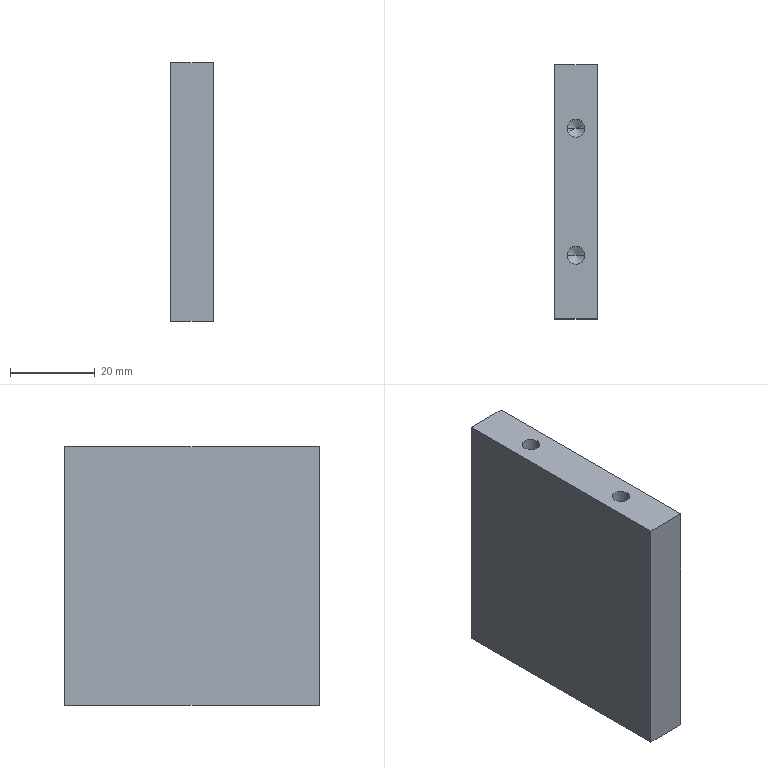Part | STEP file | 0232_207_Plate | 1 solid | 22 faces | box 10 x 60 x 61 mm | volume 35801 mm3 | cylinder 8 | cone 8 | plane 6 | commonest cylinder face diameters 4.2 x8
STEP:
#1=CARTESIAN_POINT('',(0.,0.,0.));
#2=DIRECTION('',(0.,0.,1.));
#3=DIRECTION('',(1.,0.,0.));
#4=AXIS2_PLACEMENT_3D('',#1,#2,#3);
#5=CARTESIAN_POINT('',(-7.1,15.,14.));
#6=VERTEX_POINT('',#5);
#7=CARTESIAN_POINT('',(-7.1,15.,0.));
#8=VERTEX_POINT('',#7);
#9=CARTESIAN_POINT('',(-7.1,15.,0.));
#10=DIRECTION('',(0.,0.,-1.));
#11=VECTOR('',#10,1.);
#12=LINE('',#9,#11);
#13=CARTESIAN_POINT('',(-5.,15.,0.));
#14=DIRECTION('',(0.,0.,-1.));
#15=DIRECTION('',(-1.,0.,0.));
#16=AXIS2_PLACEMENT_3D('',#13,#14,#15);
#17=CYLINDRICAL_SURFACE('',#16,2.1);
#18=CARTESIAN_POINT('',(6.283,0.));
#19=DIRECTION('',(0.,1.));
#20=VECTOR('',#19,1.);
#21=LINE('',#18,#20);
#22=(GEOMETRIC_REPRESENTATION_CONTEXT(2)PARAMETRIC_REPRESENTATION_CONTEXT()REPRESENTATION_CONTEXT('',''));
#23=DEFINITIONAL_REPRESENTATION('',(#21),#22);
#24=PCURVE('',#17,#23);
#25=CARTESIAN_POINT('',(-5.,15.,0.));
#26=DIRECTION('',(0.,0.,-1.));
#27=DIRECTION('',(-1.,0.,0.));
#28=AXIS2_PLACEMENT_3D('',#25,#26,#27);
#29=CYLINDRICAL_SURFACE('',#28,2.1);
#30=CARTESIAN_POINT('',(0.,0.));
#31=DIRECTION('',(0.,1.));
#32=VECTOR('',#31,1.);
#33=LINE('',#30,#32);
#34=(GEOMETRIC_REPRESENTATION_CONTEXT(2)PARAMETRIC_REPRESENTATION_CONTEXT()REPRESENTATION_CONTEXT('',''));
#35=DEFINITIONAL_REPRESENTATION('',(#33),#34);
#36=PCURVE('',#29,#35);
#37=SURFACE_CURVE('',#12,(#24,#36),.PCURVE_S1.);
#38=EDGE_CURVE('',#6,#8,#37,.T.);
#39=ORIENTED_EDGE('',*,*,#38,.T.);
#40=CARTESIAN_POINT('',(-2.9,15.,0.));
#41=VERTEX_POINT('',#40);
#42=CARTESIAN_POINT('',(-5.,15.,0.));
#43=DIRECTION('',(0.,0.,-1.));
#44=DIRECTION('',(-1.,0.,0.));
#45=AXIS2_PLACEMENT_3D('',#42,#43,#44);
#46=CIRCLE('',#45,2.1);
#47=CARTESIAN_POINT('',(0.,0.));
#48=DIRECTION('',(1.,0.));
#49=VECTOR('',#48,1.);
#50=LINE('',#47,#49);
#51=(GEOMETRIC_REPRESENTATION_CONTEXT(2)PARAMETRIC_REPRESENTATION_CONTEXT()REPRESENTATION_CONTEXT('',''));
#52=DEFINITIONAL_REPRESENTATION('',(#50),#51);
#53=PCURVE('',#17,#52);
#54=CARTESIAN_POINT('',(-10.,30.,0.));
#55=DIRECTION('',(0.,0.,-1.));
#56=DIRECTION('',(-1.,0.,0.));
#57=AXIS2_PLACEMENT_3D('',#54,#55,#56);
#58=PLANE('',#57);
#59=CARTESIAN_POINT('',(-5.,-15.));
#60=DIRECTION('',(1.,0.));
#61=AXIS2_PLACEMENT_2D('',#59,#60);
#62=CIRCLE('',#61,2.1);
#63=(GEOMETRIC_REPRESENTATION_CONTEXT(2)PARAMETRIC_REPRESENTATION_CONTEXT()REPRESENTATION_CONTEXT('',''));
#64=DEFINITIONAL_REPRESENTATION('',(#62),#63);
#65=PCURVE('',#58,#64);
#66=SURFACE_CURVE('',#46,(#53,#65),.PCURVE_S1.);
#67=EDGE_CURVE('',#41,#8,#66,.T.);
#68=ORIENTED_EDGE('',*,*,#67,.F.);
#69=CARTESIAN_POINT('',(-2.9,15.,14.));
#70=VERTEX_POINT('',#69);
#71=CARTESIAN_POINT('',(-2.9,15.,0.));
#72=DIRECTION('',(0.,0.,-1.));
#73=VECTOR('',#72,1.);
#74=LINE('',#71,#73);
#75=CARTESIAN_POINT('',(3.142,0.));
#76=DIRECTION('',(0.,1.));
#77=VECTOR('',#76,1.);
#78=LINE('',#75,#77);
#79=(GEOMETRIC_REPRESENTATION_CONTEXT(2)PARAMETRIC_REPRESENTATION_CONTEXT()REPRESENTATION_CONTEXT('',''));
#80=DEFINITIONAL_REPRESENTATION('',(#78),#79);
#81=PCURVE('',#17,#80);
#82=CARTESIAN_POINT('',(3.142,0.));
#83=DIRECTION('',(0.,1.));
#84=VECTOR('',#83,1.);
#85=LINE('',#82,#84);
#86=(GEOMETRIC_REPRESENTATION_CONTEXT(2)PARAMETRIC_REPRESENTATION_CONTEXT()REPRESENTATION_CONTEXT('',''));
#87=DEFINITIONAL_REPRESENTATION('',(#85),#86);
#88=PCURVE('',#29,#87);
#89=SURFACE_CURVE('',#74,(#81,#88),.PCURVE_S1.);
#90=EDGE_CURVE('',#70,#41,#89,.T.);
#91=ORIENTED_EDGE('',*,*,#90,.F.);
#92=CARTESIAN_POINT('',(-5.,15.,14.));
#93=DIRECTION('',(0.,0.,-1.));
#94=DIRECTION('',(-1.,0.,0.));
#95=AXIS2_PLACEMENT_3D('',#92,#93,#94);
#96=CIRCLE('',#95,2.1);
#97=CARTESIAN_POINT('',(0.,-14.));
#98=DIRECTION('',(1.,0.));
#99=VECTOR('',#98,1.);
#100=LINE('',#97,#99);
#101=(GEOMETRIC_REPRESENTATION_CONTEXT(2)PARAMETRIC_REPRESENTATION_CONTEXT()REPRESENTATION_CONTEXT('',''));
#102=DEFINITIONAL_REPRESENTATION('',(#100),#101);
#103=PCURVE('',#17,#102);
#104=CARTESIAN_POINT('',(-5.,15.,14.));
#105=DIRECTION('',(0.,0.,-1.));
#106=DIRECTION('',(-1.,0.,0.));
#107=AXIS2_PLACEMENT_3D('',#104,#105,#106);
#108=CONICAL_SURFACE('',#107,2.1,1.03);
#109=CARTESIAN_POINT('',(0.,0.));
#110=DIRECTION('',(1.,0.));
#111=VECTOR('',#110,1.);
#112=LINE('',#109,#111);
#113=(GEOMETRIC_REPRESENTATION_CONTEXT(2)PARAMETRIC_REPRESENTATION_CONTEXT()REPRESENTATION_CONTEXT('',''));
#114=DEFINITIONAL_REPRESENTATION('',(#112),#113);
#115=PCURVE('',#108,#114);
#116=SURFACE_CURVE('',#96,(#103,#115),.PCURVE_S1.);
#117=EDGE_CURVE('',#70,#6,#116,.T.);
#118=ORIENTED_EDGE('',*,*,#117,.T.);
#119=EDGE_LOOP('',(#39,#68,#91,#118));
#120=FACE_BOUND('',#119,.F.);
#121=ADVANCED_FACE('',(#120),#17,.F.);
#122=ORIENTED_EDGE('',*,*,#117,.F.);
#123=CARTESIAN_POINT('',(-5.,15.,15.262));
#124=VERTEX_POINT('',#123);
#125=CARTESIAN_POINT('',(-2.9,15.,14.));
#126=DIRECTION('',(0.8572,0.,-0.515));
#127=VECTOR('',#126,1.);
#128=LINE('',#125,#127);
#129=CARTESIAN_POINT('',(3.142,0.));
#130=DIRECTION('',(0.,1.));
#131=VECTOR('',#130,1.);
#132=LINE('',#129,#131);
#133=(GEOMETRIC_REPRESENTATION_CONTEXT(2)PARAMETRIC_REPRESENTATION_CONTEXT()REPRESENTATION_CONTEXT('',''));
#134=DEFINITIONAL_REPRESENTATION('',(#132),#133);
#135=PCURVE('',#108,#134);
#136=CARTESIAN_POINT('',(-5.,15.,14.));
#137=DIRECTION('',(0.,0.,-1.));
#138=DIRECTION('',(-1.,0.,0.));
#139=AXIS2_PLACEMENT_3D('',#136,#137,#138);
#140=CONICAL_SURFACE('',#139,2.1,1.03);
#141=CARTESIAN_POINT('',(3.142,0.));
#142=DIRECTION('',(0.,1.));
#143=VECTOR('',#142,1.);
#144=LINE('',#141,#143);
#145=(GEOMETRIC_REPRESENTATION_CONTEXT(2)PARAMETRIC_REPRESENTATION_CONTEXT()REPRESENTATION_CONTEXT('',''));
#146=DEFINITIONAL_REPRESENTATION('',(#144),#145);
#147=PCURVE('',#140,#146);
#148=SURFACE_CURVE('',#128,(#135,#147),.PCURVE_S1.);
#149=EDGE_CURVE('',#124,#70,#148,.T.);
#150=ORIENTED_EDGE('',*,*,#149,.F.);
#151=CARTESIAN_POINT('',(-7.1,15.,14.));
#152=DIRECTION('',(-0.8572,0.,-0.515));
#153=VECTOR('',#152,1.);
#154=LINE('',#151,#153);
#155=CARTESIAN_POINT('',(6.283,0.));
#156=DIRECTION('',(0.,1.));
#157=VECTOR('',#156,1.);
#158=LINE('',#155,#157);
#159=(GEOMETRIC_REPRESENTATION_CONTEXT(2)PARAMETRIC_REPRESENTATION_CONTEXT()REPRESENTATION_CONTEXT('',''));
#160=DEFINITIONAL_REPRESENTATION('',(#158),#159);
#161=PCURVE('',#108,#160);
#162=CARTESIAN_POINT('',(0.,0.));
#163=DIRECTION('',(0.,1.));
#164=VECTOR('',#163,1.);
#165=LINE('',#162,#164);
#166=(GEOMETRIC_REPRESENTATION_CONTEXT(2)PARAMETRIC_REPRESENTATION_CONTEXT()REPRESENTATION_CONTEXT('',''));
#167=DEFINITIONAL_REPRESENTATION('',(#165),#166);
#168=PCURVE('',#140,#167);
#169=SURFACE_CURVE('',#154,(#161,#168),.PCURVE_S1.);
#170=EDGE_CURVE('',#124,#6,#169,.T.);
#171=ORIENTED_EDGE('',*,*,#170,.T.);
#172=EDGE_LOOP('',(#122,#150,#171));
#173=FACE_BOUND('',#172,.F.);
#174=ADVANCED_FACE('',(#173),#108,.F.);
#175=CARTESIAN_POINT('',(-7.1,-15.,14.));
#176=VERTEX_POINT('',#175);
#177=CARTESIAN_POINT('',(-7.1,-15.,0.));
#178=VERTEX_POINT('',#177);
#179=CARTESIAN_POINT('',(-7.1,-15.,0.));
#180=DIRECTION('',(0.,0.,-1.));
#181=VECTOR('',#180,1.);
#182=LINE('',#179,#181);
#183=CARTESIAN_POINT('',(-5.,-15.,0.));
#184=DIRECTION('',(0.,0.,-1.));
#185=DIRECTION('',(-1.,0.,0.));
#186=AXIS2_PLACEMENT_3D('',#183,#184,#185);
#187=CYLINDRICAL_SURFACE('',#186,2.1);
#188=CARTESIAN_POINT('',(6.283,0.));
#189=DIRECTION('',(0.,1.));
#190=VECTOR('',#189,1.);
#191=LINE('',#188,#190);
#192=(GEOMETRIC_REPRESENTATION_CONTEXT(2)PARAMETRIC_REPRESENTATION_CONTEXT()REPRESENTATION_CONTEXT('',''));
#193=DEFINITIONAL_REPRESENTATION('',(#191),#192);
#194=PCURVE('',#187,#193);
#195=CARTESIAN_POINT('',(-5.,-15.,0.));
#196=DIRECTION('',(0.,0.,-1.));
#197=DIRECTION('',(-1.,0.,0.));
#198=AXIS2_PLACEMENT_3D('',#195,#196,#197);
#199=CYLINDRICAL_SURFACE('',#198,2.1);
#200=CARTESIAN_POINT('',(0.,0.));
#201=DIRECTION('',(0.,1.));
#202=VECTOR('',#201,1.);
#203=LINE('',#200,#202);
#204=(GEOMETRIC_REPRESENTATION_CONTEXT(2)PARAMETRIC_REPRESENTATION_CONTEXT()REPRESENTATION_CONTEXT('',''));
#205=DEFINITIONAL_REPRESENTATION('',(#203),#204);
#206=PCURVE('',#199,#205);
#207=SURFACE_CURVE('',#182,(#194,#206),.PCURVE_S1.);
#208=EDGE_CURVE('',#176,#178,#207,.T.);
#209=ORIENTED_EDGE('',*,*,#208,.T.);
#210=CARTESIAN_POINT('',(-2.9,-15.,0.));
#211=VERTEX_POINT('',#210);
#212=CARTESIAN_POINT('',(-5.,-15.,0.));
#213=DIRECTION('',(0.,0.,-1.));
#214=DIRECTION('',(-1.,0.,0.));
#215=AXIS2_PLACEMENT_3D('',#212,#213,#214);
#216=CIRCLE('',#215,2.1);
#217=CARTESIAN_POINT('',(0.,0.));
#218=DIRECTION('',(1.,0.));
#219=VECTOR('',#218,1.);
#220=LINE('',#217,#219);
#221=(GEOMETRIC_REPRESENTATION_CONTEXT(2)PARAMETRIC_REPRESENTATION_CONTEXT()REPRESENTATION_CONTEXT('',''));
#222=DEFINITIONAL_REPRESENTATION('',(#220),#221);
#223=PCURVE('',#187,#222);
#224=CARTESIAN_POINT('',(-5.,-45.));
#225=DIRECTION('',(1.,0.));
#226=AXIS2_PLACEMENT_2D('',#224,#225);
#227=CIRCLE('',#226,2.1);
#228=(GEOMETRIC_REPRESENTATION_CONTEXT(2)PARAMETRIC_REPRESENTATION_CONTEXT()REPRESENTATION_CONTEXT('',''));
#229=DEFINITIONAL_REPRESENTATION('',(#227),#228);
#230=PCURVE('',#58,#229);
#231=SURFACE_CURVE('',#216,(#223,#230),.PCURVE_S1.);
#232=EDGE_CURVE('',#211,#178,#231,.T.);
#233=ORIENTED_EDGE('',*,*,#232,.F.);
#234=CARTESIAN_POINT('',(-2.9,-15.,14.));
#235=VERTEX_POINT('',#234);
#236=CARTESIAN_POINT('',(-2.9,-15.,0.));
#237=DIRECTION('',(0.,0.,-1.));
#238=VECTOR('',#237,1.);
#239=LINE('',#236,#238);
#240=CARTESIAN_POINT('',(3.142,0.));
#241=DIRECTION('',(0.,1.));
#242=VECTOR('',#241,1.);
#243=LINE('',#240,#242);
#244=(GEOMETRIC_REPRESENTATION_CONTEXT(2)PARAMETRIC_REPRESENTATION_CONTEXT()REPRESENTATION_CONTEXT('',''));
#245=DEFINITIONAL_REPRESENTATION('',(#243),#244);
#246=PCURVE('',#187,#245);
#247=CARTESIAN_POINT('',(3.142,0.));
#248=DIRECTION('',(0.,1.));
#249=VECTOR('',#248,1.);
#250=LINE('',#247,#249);
#251=(GEOMETRIC_REPRESENTATION_CONTEXT(2)PARAMETRIC_REPRESENTATION_CONTEXT()REPRESENTATION_CONTEXT('',''));
#252=DEFINITIONAL_REPRESENTATION('',(#250),#251);
#253=PCURVE('',#199,#252);
#254=SURFACE_CURVE('',#239,(#246,#253),.PCURVE_S1.);
#255=EDGE_CURVE('',#235,#211,#254,.T.);
#256=ORIENTED_EDGE('',*,*,#255,.F.);
#257=CARTESIAN_POINT('',(-5.,-15.,14.));
#258=DIRECTION('',(0.,0.,-1.));
#259=DIRECTION('',(-1.,0.,0.));
#260=AXIS2_PLACEMENT_3D('',#257,#258,#259);
#261=CIRCLE('',#260,2.1);
#262=CARTESIAN_POINT('',(0.,-14.));
#263=DIRECTION('',(1.,0.));
#264=VECTOR('',#263,1.);
#265=LINE('',#262,#264);
#266=(GEOMETRIC_REPRESENTATION_CONTEXT(2)PARAMETRIC_REPRESENTATION_CONTEXT()REPRESENTATION_CONTEXT('',''));
#267=DEFINITIONAL_REPRESENTATION('',(#265),#266);
#268=PCURVE('',#187,#267);
#269=CARTESIAN_POINT('',(-5.,-15.,14.));
#270=DIRECTION('',(0.,0.,-1.));
#271=DIRECTION('',(-1.,0.,0.));
#272=AXIS2_PLACEMENT_3D('',#269,#270,#271);
#273=CONICAL_SURFACE('',#272,2.1,1.03);
#274=CARTESIAN_POINT('',(0.,0.));
#275=DIRECTION('',(1.,0.));
#276=VECTOR('',#275,1.);
#277=LINE('',#274,#276);
#278=(GEOMETRIC_REPRESENTATION_CONTEXT(2)PARAMETRIC_REPRESENTATION_CONTEXT()REPRESENTATION_CONTEXT('',''));
#279=DEFINITIONAL_REPRESENTATION('',(#277),#278);
#280=PCURVE('',#273,#279);
#281=SURFACE_CURVE('',#261,(#268,#280),.PCURVE_S1.);
#282=EDGE_CURVE('',#235,#176,#281,.T.);
#283=ORIENTED_EDGE('',*,*,#282,.T.);
#284=EDGE_LOOP('',(#209,#233,#256,#283));
#285=FACE_BOUND('',#284,.F.);
#286=ADVANCED_FACE('',(#285),#187,.F.);
#287=ORIENTED_EDGE('',*,*,#282,.F.);
#288=CARTESIAN_POINT('',(-5.,-15.,15.262));
#289=VERTEX_POINT('',#288);
#290=CARTESIAN_POINT('',(-2.9,-15.,14.));
#291=DIRECTION('',(0.8572,0.,-0.515));
#292=VECTOR('',#291,1.);
#293=LINE('',#290,#292);
#294=CARTESIAN_POINT('',(3.142,0.));
#295=DIRECTION('',(0.,1.));
#296=VECTOR('',#295,1.);
#297=LINE('',#294,#296);
#298=(GEOMETRIC_REPRESENTATION_CONTEXT(2)PARAMETRIC_REPRESENTATION_CONTEXT()REPRESENTATION_CONTEXT('',''));
#299=DEFINITIONAL_REPRESENTATION('',(#297),#298);
#300=PCURVE('',#273,#299);
#301=CARTESIAN_POINT('',(-5.,-15.,14.));
#302=DIRECTION('',(0.,0.,-1.));
#303=DIRECTION('',(-1.,0.,0.));
#304=AXIS2_PLACEMENT_3D('',#301,#302,#303);
#305=CONICAL_SURFACE('',#304,2.1,1.03);
#306=CARTESIAN_POINT('',(3.142,0.));
#307=DIRECTION('',(0.,1.));
#308=VECTOR('',#307,1.);
#309=LINE('',#306,#308);
#310=(GEOMETRIC_REPRESENTATION_CONTEXT(2)PARAMETRIC_REPRESENTATION_CONTEXT()REPRESENTATION_CONTEXT('',''));
#311=DEFINITIONAL_REPRESENTATION('',(#309),#310);
#312=PCURVE('',#305,#311);
#313=SURFACE_CURVE('',#293,(#300,#312),.PCURVE_S1.);
#314=EDGE_CURVE('',#289,#235,#313,.T.);
#315=ORIENTED_EDGE('',*,*,#314,.F.);
#316=CARTESIAN_POINT('',(-7.1,-15.,14.));
#317=DIRECTION('',(-0.8572,0.,-0.515));
#318=VECTOR('',#317,1.);
#319=LINE('',#316,#318);
#320=CARTESIAN_POINT('',(6.283,0.));
#321=DIRECTION('',(0.,1.));
#322=VECTOR('',#321,1.);
#323=LINE('',#320,#322);
#324=(GEOMETRIC_REPRESENTATION_CONTEXT(2)PARAMETRIC_REPRESENTATION_CONTEXT()REPRESENTATION_CONTEXT('',''));
#325=DEFINITIONAL_REPRESENTATION('',(#323),#324);
#326=PCURVE('',#273,#325);
#327=CARTESIAN_POINT('',(0.,0.));
#328=DIRECTION('',(0.,1.));
#329=VECTOR('',#328,1.);
#330=LINE('',#327,#329);
#331=(GEOMETRIC_REPRESENTATION_CONTEXT(2)PARAMETRIC_REPRESENTATION_CONTEXT()REPRESENTATION_CONTEXT('',''));
#332=DEFINITIONAL_REPRESENTATION('',(#330),#331);
#333=PCURVE('',#305,#332);
#334=SURFACE_CURVE('',#319,(#326,#333),.PCURVE_S1.);
#335=EDGE_CURVE('',#289,#176,#334,.T.);
#336=ORIENTED_EDGE('',*,*,#335,.T.);
#337=EDGE_LOOP('',(#287,#315,#336));
#338=FACE_BOUND('',#337,.F.);
#339=ADVANCED_FACE('',(#338),#273,.F.);
#340=CARTESIAN_POINT('',(-2.9,-15.,47.));
#341=VERTEX_POINT('',#340);
#342=CARTESIAN_POINT('',(-2.9,-15.,61.));
#343=VERTEX_POINT('',#342);
#344=CARTESIAN_POINT('',(-2.9,-15.,61.));
#345=DIRECTION('',(0.,0.,1.));
#346=VECTOR('',#345,1.);
#347=LINE('',#344,#346);
#348=CARTESIAN_POINT('',(-5.,-15.,61.));
#349=DIRECTION('',(0.,0.,1.));
#350=DIRECTION('',(1.,0.,0.));
#351=AXIS2_PLACEMENT_3D('',#348,#349,#350);
#352=CYLINDRICAL_SURFACE('',#351,2.1);
#353=CARTESIAN_POINT('',(6.283,0.));
#354=DIRECTION('',(0.,1.));
#355=VECTOR('',#354,1.);
#356=LINE('',#353,#355);
#357=(GEOMETRIC_REPRESENTATION_CONTEXT(2)PARAMETRIC_REPRESENTATION_CONTEXT()REPRESENTATION_CONTEXT('',''));
#358=DEFINITIONAL_REPRESENTATION('',(#356),#357);
#359=PCURVE('',#352,#358);
#360=CARTESIAN_POINT('',(-5.,-15.,61.));
#361=DIRECTION('',(0.,0.,1.));
#362=DIRECTION('',(1.,0.,0.));
#363=AXIS2_PLACEMENT_3D('',#360,#361,#362);
#364=CYLINDRICAL_SURFACE('',#363,2.1);
#365=CARTESIAN_POINT('',(0.,0.));
#366=DIRECTION('',(0.,1.));
#367=VECTOR('',#366,1.);
#368=LINE('',#365,#367);
#369=(GEOMETRIC_REPRESENTATION_CONTEXT(2)PARAMETRIC_REPRESENTATION_CONTEXT()REPRESENTATION_CONTEXT('',''));
#370=DEFINITIONAL_REPRESENTATION('',(#368),#369);
#371=PCURVE('',#364,#370);
#372=SURFACE_CURVE('',#347,(#359,#371),.PCURVE_S1.);
#373=EDGE_CURVE('',#341,#343,#372,.T.);
#374=ORIENTED_EDGE('',*,*,#373,.T.);
#375=CARTESIAN_POINT('',(-7.1,-15.,61.));
#376=VERTEX_POINT('',#375);
#377=CARTESIAN_POINT('',(-5.,-15.,61.));
#378=DIRECTION('',(0.,0.,1.));
#379=DIRECTION('',(1.,0.,0.));
#380=AXIS2_PLACEMENT_3D('',#377,#378,#379);
#381=CIRCLE('',#380,2.1);
#382=CARTESIAN_POINT('',(0.,0.));
#383=DIRECTION('',(1.,0.));
#384=VECTOR('',#383,1.);
#385=LINE('',#382,#384);
#386=(GEOMETRIC_REPRESENTATION_CONTEXT(2)PARAMETRIC_REPRESENTATION_CONTEXT()REPRESENTATION_CONTEXT('',''));
#387=DEFINITIONAL_REPRESENTATION('',(#385),#386);
#388=PCURVE('',#352,#387);
#389=CARTESIAN_POINT('',(-10.,30.,61.));
#390=DIRECTION('',(0.,0.,1.));
#391=DIRECTION('',(1.,0.,0.));
#392=AXIS2_PLACEMENT_3D('',#389,#390,#391);
#393=PLANE('',#392);
#394=CARTESIAN_POINT('',(5.,-45.));
#395=DIRECTION('',(1.,0.));
#396=AXIS2_PLACEMENT_2D('',#394,#395);
#397=CIRCLE('',#396,2.1);
#398=(GEOMETRIC_REPRESENTATION_CONTEXT(2)PARAMETRIC_REPRESENTATION_CONTEXT()REPRESENTATION_CONTEXT('',''));
#399=DEFINITIONAL_REPRESENTATION('',(#397),#398);
#400=PCURVE('',#393,#399);
#401=SURFACE_CURVE('',#381,(#388,#400),.PCURVE_S1.);
#402=EDGE_CURVE('',#376,#343,#401,.T.);
#403=ORIENTED_EDGE('',*,*,#402,.F.);
#404=CARTESIAN_POINT('',(-7.1,-15.,47.));
#405=VERTEX_POINT('',#404);
#406=CARTESIAN_POINT('',(-7.1,-15.,61.));
#407=DIRECTION('',(0.,0.,1.));
#408=VECTOR('',#407,1.);
#409=LINE('',#406,#408);
#410=CARTESIAN_POINT('',(3.142,0.));
#411=DIRECTION('',(0.,1.));
#412=VECTOR('',#411,1.);
#413=LINE('',#410,#412);
#414=(GEOMETRIC_REPRESENTATION_CONTEXT(2)PARAMETRIC_REPRESENTATION_CONTEXT()REPRESENTATION_CONTEXT('',''));
#415=DEFINITIONAL_REPRESENTATION('',(#413),#414);
#416=PCURVE('',#352,#415);
#417=CARTESIAN_POINT('',(3.142,0.));
#418=DIRECTION('',(0.,1.));
#419=VECTOR('',#418,1.);
#420=LINE('',#417,#419);
#421=(GEOMETRIC_REPRESENTATION_CONTEXT(2)PARAMETRIC_REPRESENTATION_CONTEXT()REPRESENTATION_CONTEXT('',''));
#422=DEFINITIONAL_REPRESENTATION('',(#420),#421);
#423=PCURVE('',#364,#422);
#424=SURFACE_CURVE('',#409,(#416,#423),.PCURVE_S1.);
#425=EDGE_CURVE('',#405,#376,#424,.T.);
#426=ORIENTED_EDGE('',*,*,#425,.F.);
#427=CARTESIAN_POINT('',(-5.,-15.,47.));
#428=DIRECTION('',(0.,0.,1.));
#429=DIRECTION('',(1.,0.,0.));
#430=AXIS2_PLACEMENT_3D('',#427,#428,#429);
#431=CIRCLE('',#430,2.1);
#432=CARTESIAN_POINT('',(0.,-14.));
#433=DIRECTION('',(1.,0.));
#434=VECTOR('',#433,1.);
#435=LINE('',#432,#434);
#436=(GEOMETRIC_REPRESENTATION_CONTEXT(2)PARAMETRIC_REPRESENTATION_CONTEXT()REPRESENTATION_CONTEXT('',''));
#437=DEFINITIONAL_REPRESENTATION('',(#435),#436);
#438=PCURVE('',#352,#437);
#439=CARTESIAN_POINT('',(-5.,-15.,47.));
#440=DIRECTION('',(0.,0.,1.));
#441=DIRECTION('',(1.,0.,0.));
#442=AXIS2_PLACEMENT_3D('',#439,#440,#441);
#443=CONICAL_SURFACE('',#442,2.1,1.03);
#444=CARTESIAN_POINT('',(0.,0.));
#445=DIRECTION('',(1.,0.));
#446=VECTOR('',#445,1.);
#447=LINE('',#444,#446);
#448=(GEOMETRIC_REPRESENTATION_CONTEXT(2)PARAMETRIC_REPRESENTATION_CONTEXT()REPRESENTATION_CONTEXT('',''));
#449=DEFINITIONAL_REPRESENTATION('',(#447),#448);
#450=PCURVE('',#443,#449);
#451=SURFACE_CURVE('',#431,(#438,#450),.PCURVE_S1.);
#452=EDGE_CURVE('',#405,#341,#451,.T.);
#453=ORIENTED_EDGE('',*,*,#452,.T.);
#454=EDGE_LOOP('',(#374,#403,#426,#453));
#455=FACE_BOUND('',#454,.F.);
#456=ADVANCED_FACE('',(#455),#352,.F.);
#457=ORIENTED_EDGE('',*,*,#452,.F.);
#458=CARTESIAN_POINT('',(-5.,-15.,45.738));
#459=VERTEX_POINT('',#458);
#460=CARTESIAN_POINT('',(-7.1,-15.,47.));
#461=DIRECTION('',(-0.8572,0.,0.515));
#462=VECTOR('',#461,1.);
#463=LINE('',#460,#462);
#464=CARTESIAN_POINT('',(3.142,0.));
#465=DIRECTION('',(0.,1.));
#466=VECTOR('',#465,1.);
#467=LINE('',#464,#466);
#468=(GEOMETRIC_REPRESENTATION_CONTEXT(2)PARAMETRIC_REPRESENTATION_CONTEXT()REPRESENTATION_CONTEXT('',''));
#469=DEFINITIONAL_REPRESENTATION('',(#467),#468);
#470=PCURVE('',#443,#469);
#471=CARTESIAN_POINT('',(-5.,-15.,47.));
#472=DIRECTION('',(0.,0.,1.));
#473=DIRECTION('',(1.,0.,0.));
#474=AXIS2_PLACEMENT_3D('',#471,#472,#473);
#475=CONICAL_SURFACE('',#474,2.1,1.03);
#476=CARTESIAN_POINT('',(3.142,0.));
#477=DIRECTION('',(0.,1.));
#478=VECTOR('',#477,1.);
#479=LINE('',#476,#478);
#480=(GEOMETRIC_REPRESENTATION_CONTEXT(2)PARAMETRIC_REPRESENTATION_CONTEXT()REPRESENTATION_CONTEXT('',''));
#481=DEFINITIONAL_REPRESENTATION('',(#479),#480);
#482=PCURVE('',#475,#481);
#483=SURFACE_CURVE('',#463,(#470,#482),.PCURVE_S1.);
#484=EDGE_CURVE('',#459,#405,#483,.T.);
#485=ORIENTED_EDGE('',*,*,#484,.F.);
#486=CARTESIAN_POINT('',(-2.9,-15.,47.));
#487=DIRECTION('',(0.8572,0.,0.515));
#488=VECTOR('',#487,1.);
#489=LINE('',#486,#488);
#490=CARTESIAN_POINT('',(6.283,0.));
#491=DIRECTION('',(0.,1.));
#492=VECTOR('',#491,1.);
#493=LINE('',#490,#492);
#494=(GEOMETRIC_REPRESENTATION_CONTEXT(2)PARAMETRIC_REPRESENTATION_CONTEXT()REPRESENTATION_CONTEXT('',''));
#495=DEFINITIONAL_REPRESENTATION('',(#493),#494);
#496=PCURVE('',#443,#495);
#497=CARTESIAN_POINT('',(0.,0.));
#498=DIRECTION('',(0.,1.));
#499=VECTOR('',#498,1.);
#500=LINE('',#497,#499);
#501=(GEOMETRIC_REPRESENTATION_CONTEXT(2)PARAMETRIC_REPRESENTATION_CONTEXT()REPRESENTATION_CONTEXT('',''));
#502=DEFINITIONAL_REPRESENTATION('',(#500),#501);
#503=PCURVE('',#475,#502);
#504=SURFACE_CURVE('',#489,(#496,#503),.PCURVE_S1.);
#505=EDGE_CURVE('',#459,#341,#504,.T.);
#506=ORIENTED_EDGE('',*,*,#505,.T.);
#507=EDGE_LOOP('',(#457,#485,#506));
#508=FACE_BOUND('',#507,.F.);
#509=ADVANCED_FACE('',(#508),#443,.F.);
#510=CARTESIAN_POINT('',(-2.9,15.,47.));
#511=VERTEX_POINT('',#510);
#512=CARTESIAN_POINT('',(-2.9,15.,61.));
#513=VERTEX_POINT('',#512);
#514=CARTESIAN_POINT('',(-2.9,15.,61.));
#515=DIRECTION('',(0.,0.,1.));
#516=VECTOR('',#515,1.);
#517=LINE('',#514,#516);
#518=CARTESIAN_POINT('',(-5.,15.,61.));
#519=DIRECTION('',(0.,0.,1.));
#520=DIRECTION('',(1.,0.,0.));
#521=AXIS2_PLACEMENT_3D('',#518,#519,#520);
#522=CYLINDRICAL_SURFACE('',#521,2.1);
#523=CARTESIAN_POINT('',(6.283,0.));
#524=DIRECTION('',(0.,1.));
#525=VECTOR('',#524,1.);
#526=LINE('',#523,#525);
#527=(GEOMETRIC_REPRESENTATION_CONTEXT(2)PARAMETRIC_REPRESENTATION_CONTEXT()REPRESENTATION_CONTEXT('',''));
#528=DEFINITIONAL_REPRESENTATION('',(#526),#527);
#529=PCURVE('',#522,#528);
#530=CARTESIAN_POINT('',(-5.,15.,61.));
#531=DIRECTION('',(0.,0.,1.));
#532=DIRECTION('',(1.,0.,0.));
#533=AXIS2_PLACEMENT_3D('',#530,#531,#532);
#534=CYLINDRICAL_SURFACE('',#533,2.1);
#535=CARTESIAN_POINT('',(0.,0.));
#536=DIRECTION('',(0.,1.));
#537=VECTOR('',#536,1.);
#538=LINE('',#535,#537);
#539=(GEOMETRIC_REPRESENTATION_CONTEXT(2)PARAMETRIC_REPRESENTATION_CONTEXT()REPRESENTATION_CONTEXT('',''));
#540=DEFINITIONAL_REPRESENTATION('',(#538),#539);
#541=PCURVE('',#534,#540);
#542=SURFACE_CURVE('',#517,(#529,#541),.PCURVE_S1.);
#543=EDGE_CURVE('',#511,#513,#542,.T.);
#544=ORIENTED_EDGE('',*,*,#543,.T.);
#545=CARTESIAN_POINT('',(-7.1,15.,61.));
#546=VERTEX_POINT('',#545);
#547=CARTESIAN_POINT('',(-5.,15.,61.));
#548=DIRECTION('',(0.,0.,1.));
#549=DIRECTION('',(1.,0.,0.));
#550=AXIS2_PLACEMENT_3D('',#547,#548,#549);
#551=CIRCLE('',#550,2.1);
#552=CARTESIAN_POINT('',(0.,0.));
#553=DIRECTION('',(1.,0.));
#554=VECTOR('',#553,1.);
#555=LINE('',#552,#554);
#556=(GEOMETRIC_REPRESENTATION_CONTEXT(2)PARAMETRIC_REPRESENTATION_CONTEXT()REPRESENTATION_CONTEXT('',''));
#557=DEFINITIONAL_REPRESENTATION('',(#555),#556);
#558=PCURVE('',#522,#557);
#559=CARTESIAN_POINT('',(5.,-15.));
#560=DIRECTION('',(1.,0.));
#561=AXIS2_PLACEMENT_2D('',#559,#560);
#562=CIRCLE('',#561,2.1);
#563=(GEOMETRIC_REPRESENTATION_CONTEXT(2)PARAMETRIC_REPRESENTATION_CONTEXT()REPRESENTATION_CONTEXT('',''));
#564=DEFINITIONAL_REPRESENTATION('',(#562),#563);
#565=PCURVE('',#393,#564);
#566=SURFACE_CURVE('',#551,(#558,#565),.PCURVE_S1.);
#567=EDGE_CURVE('',#546,#513,#566,.T.);
#568=ORIENTED_EDGE('',*,*,#567,.F.);
#569=CARTESIAN_POINT('',(-7.1,15.,47.));
#570=VERTEX_POINT('',#569);
#571=CARTESIAN_POINT('',(-7.1,15.,61.));
#572=DIRECTION('',(0.,0.,1.));
#573=VECTOR('',#572,1.);
#574=LINE('',#571,#573);
#575=CARTESIAN_POINT('',(3.142,0.));
#576=DIRECTION('',(0.,1.));
#577=VECTOR('',#576,1.);
#578=LINE('',#575,#577);
#579=(GEOMETRIC_REPRESENTATION_CONTEXT(2)PARAMETRIC_REPRESENTATION_CONTEXT()REPRESENTATION_CONTEXT('',''));
#580=DEFINITIONAL_REPRESENTATION('',(#578),#579);
#581=PCURVE('',#522,#580);
#582=CARTESIAN_POINT('',(3.142,0.));
#583=DIRECTION('',(0.,1.));
#584=VECTOR('',#583,1.);
#585=LINE('',#582,#584);
#586=(GEOMETRIC_REPRESENTATION_CONTEXT(2)PARAMETRIC_REPRESENTATION_CONTEXT()REPRESENTATION_CONTEXT('',''));
#587=DEFINITIONAL_REPRESENTATION('',(#585),#586);
#588=PCURVE('',#534,#587);
#589=SURFACE_CURVE('',#574,(#581,#588),.PCURVE_S1.);
#590=EDGE_CURVE('',#570,#546,#589,.T.);
#591=ORIENTED_EDGE('',*,*,#590,.F.);
#592=CARTESIAN_POINT('',(-5.,15.,47.));
#593=DIRECTION('',(0.,0.,1.));
#594=DIRECTION('',(1.,0.,0.));
#595=AXIS2_PLACEMENT_3D('',#592,#593,#594);
#596=CIRCLE('',#595,2.1);
#597=CARTESIAN_POINT('',(0.,-14.));
#598=DIRECTION('',(1.,0.));
#599=VECTOR('',#598,1.);
#600=LINE('',#597,#599);
#601=(GEOMETRIC_REPRESENTATION_CONTEXT(2)PARAMETRIC_REPRESENTATION_CONTEXT()REPRESENTATION_CONTEXT('',''));
#602=DEFINITIONAL_REPRESENTATION('',(#600),#601);
#603=PCURVE('',#522,#602);
#604=CARTESIAN_POINT('',(-5.,15.,47.));
#605=DIRECTION('',(0.,0.,1.));
#606=DIRECTION('',(1.,0.,0.));
#607=AXIS2_PLACEMENT_3D('',#604,#605,#606);
#608=CONICAL_SURFACE('',#607,2.1,1.03);
#609=CARTESIAN_POINT('',(0.,0.));
#610=DIRECTION('',(1.,0.));
#611=VECTOR('',#610,1.);
#612=LINE('',#609,#611);
#613=(GEOMETRIC_REPRESENTATION_CONTEXT(2)PARAMETRIC_REPRESENTATION_CONTEXT()REPRESENTATION_CONTEXT('',''));
#614=DEFINITIONAL_REPRESENTATION('',(#612),#613);
#615=PCURVE('',#608,#614);
#616=SURFACE_CURVE('',#596,(#603,#615),.PCURVE_S1.);
#617=EDGE_CURVE('',#570,#511,#616,.T.);
#618=ORIENTED_EDGE('',*,*,#617,.T.);
#619=EDGE_LOOP('',(#544,#568,#591,#618));
#620=FACE_BOUND('',#619,.F.);
#621=ADVANCED_FACE('',(#620),#522,.F.);
#622=ORIENTED_EDGE('',*,*,#617,.F.);
#623=CARTESIAN_POINT('',(-5.,15.,45.738));
#624=VERTEX_POINT('',#623);
#625=CARTESIAN_POINT('',(-7.1,15.,47.));
#626=DIRECTION('',(-0.8572,0.,0.515));
#627=VECTOR('',#626,1.);
#628=LINE('',#625,#627);
#629=CARTESIAN_POINT('',(3.142,0.));
#630=DIRECTION('',(0.,1.));
#631=VECTOR('',#630,1.);
#632=LINE('',#629,#631);
#633=(GEOMETRIC_REPRESENTATION_CONTEXT(2)PARAMETRIC_REPRESENTATION_CONTEXT()REPRESENTATION_CONTEXT('',''));
#634=DEFINITIONAL_REPRESENTATION('',(#632),#633);
#635=PCURVE('',#608,#634);
#636=CARTESIAN_POINT('',(-5.,15.,47.));
#637=DIRECTION('',(0.,0.,1.));
#638=DIRECTION('',(1.,0.,0.));
#639=AXIS2_PLACEMENT_3D('',#636,#637,#638);
#640=CONICAL_SURFACE('',#639,2.1,1.03);
#641=CARTESIAN_POINT('',(3.142,0.));
#642=DIRECTION('',(0.,1.));
#643=VECTOR('',#642,1.);
#644=LINE('',#641,#643);
#645=(GEOMETRIC_REPRESENTATION_CONTEXT(2)PARAMETRIC_REPRESENTATION_CONTEXT()REPRESENTATION_CONTEXT('',''));
#646=DEFINITIONAL_REPRESENTATION('',(#644),#645);
#647=PCURVE('',#640,#646);
#648=SURFACE_CURVE('',#628,(#635,#647),.PCURVE_S1.);
#649=EDGE_CURVE('',#624,#570,#648,.T.);
#650=ORIENTED_EDGE('',*,*,#649,.F.);
#651=CARTESIAN_POINT('',(-2.9,15.,47.));
#652=DIRECTION('',(0.8572,0.,0.515));
#653=VECTOR('',#652,1.);
#654=LINE('',#651,#653);
#655=CARTESIAN_POINT('',(6.283,0.));
#656=DIRECTION('',(0.,1.));
#657=VECTOR('',#656,1.);
#658=LINE('',#655,#657);
#659=(GEOMETRIC_REPRESENTATION_CONTEXT(2)PARAMETRIC_REPRESENTATION_CONTEXT()REPRESENTATION_CONTEXT('',''));
#660=DEFINITIONAL_REPRESENTATION('',(#658),#659);
#661=PCURVE('',#608,#660);
#662=CARTESIAN_POINT('',(0.,0.));
#663=DIRECTION('',(0.,1.));
#664=VECTOR('',#663,1.);
#665=LINE('',#662,#664);
#666=(GEOMETRIC_REPRESENTATION_CONTEXT(2)PARAMETRIC_REPRESENTATION_CONTEXT()REPRESENTATION_CONTEXT('',''));
#667=DEFINITIONAL_REPRESENTATION('',(#665),#666);
#668=PCURVE('',#640,#667);
#669=SURFACE_CURVE('',#654,(#661,#668),.PCURVE_S1.);
#670=EDGE_CURVE('',#624,#511,#669,.T.);
#671=ORIENTED_EDGE('',*,*,#670,.T.);
#672=EDGE_LOOP('',(#622,#650,#671));
#673=FACE_BOUND('',#672,.F.);
#674=ADVANCED_FACE('',(#673),#608,.F.);
#675=CARTESIAN_POINT('',(-5.,-15.,61.));
#676=DIRECTION('',(0.,0.,1.));
#677=DIRECTION('',(1.,0.,0.));
#678=AXIS2_PLACEMENT_3D('',#675,#676,#677);
#679=CIRCLE('',#678,2.1);
#680=CARTESIAN_POINT('',(5.,-45.));
#681=DIRECTION('',(1.,0.));
#682=AXIS2_PLACEMENT_2D('',#680,#681);
#683=CIRCLE('',#682,2.1);
#684=(GEOMETRIC_REPRESENTATION_CONTEXT(2)PARAMETRIC_REPRESENTATION_CONTEXT()REPRESENTATION_CONTEXT('',''));
#685=DEFINITIONAL_REPRESENTATION('',(#683),#684);
#686=PCURVE('',#393,#685);
#687=CARTESIAN_POINT('',(0.,0.));
#688=DIRECTION('',(1.,0.));
#689=VECTOR('',#688,1.);
#690=LINE('',#687,#689);
#691=(GEOMETRIC_REPRESENTATION_CONTEXT(2)PARAMETRIC_REPRESENTATION_CONTEXT()REPRESENTATION_CONTEXT('',''));
#692=DEFINITIONAL_REPRESENTATION('',(#690),#691);
#693=PCURVE('',#364,#692);
#694=SURFACE_CURVE('',#679,(#686,#693),.PCURVE_S1.);
#695=EDGE_CURVE('',#343,#376,#694,.T.);
#696=ORIENTED_EDGE('',*,*,#695,.F.);
#697=ORIENTED_EDGE('',*,*,#402,.F.);
#698=EDGE_LOOP('',(#696,#697));
#699=FACE_BOUND('',#698,.T.);
#700=CARTESIAN_POINT('',(-5.,15.,61.));
#701=DIRECTION('',(0.,0.,1.));
#702=DIRECTION('',(1.,0.,0.));
#703=AXIS2_PLACEMENT_3D('',#700,#701,#702);
#704=CIRCLE('',#703,2.1);
#705=CARTESIAN_POINT('',(5.,-15.));
#706=DIRECTION('',(1.,0.));
#707=AXIS2_PLACEMENT_2D('',#705,#706);
#708=CIRCLE('',#707,2.1);
#709=(GEOMETRIC_REPRESENTATION_CONTEXT(2)PARAMETRIC_REPRESENTATION_CONTEXT()REPRESENTATION_CONTEXT('',''));
#710=DEFINITIONAL_REPRESENTATION('',(#708),#709);
#711=PCURVE('',#393,#710);
#712=CARTESIAN_POINT('',(0.,0.));
#713=DIRECTION('',(1.,0.));
#714=VECTOR('',#713,1.);
#715=LINE('',#712,#714);
#716=(GEOMETRIC_REPRESENTATION_CONTEXT(2)PARAMETRIC_REPRESENTATION_CONTEXT()REPRESENTATION_CONTEXT('',''));
#717=DEFINITIONAL_REPRESENTATION('',(#715),#716);
#718=PCURVE('',#534,#717);
#719=SURFACE_CURVE('',#704,(#711,#718),.PCURVE_S1.);
#720=EDGE_CURVE('',#513,#546,#719,.T.);
#721=ORIENTED_EDGE('',*,*,#720,.F.);
#722=ORIENTED_EDGE('',*,*,#567,.F.);
#723=EDGE_LOOP('',(#721,#722));
#724=FACE_BOUND('',#723,.T.);
#725=CARTESIAN_POINT('',(0.,30.,61.));
#726=VERTEX_POINT('',#725);
#727=CARTESIAN_POINT('',(0.,-30.,61.));
#728=VERTEX_POINT('',#727);
#729=CARTESIAN_POINT('',(0.,30.,61.));
#730=DIRECTION('',(0.,-1.,0.));
#731=VECTOR('',#730,1.);
#732=LINE('',#729,#731);
#733=CARTESIAN_POINT('',(10.,0.));
#734=DIRECTION('',(0.,-1.));
#735=VECTOR('',#734,1.);
#736=LINE('',#733,#735);
#737=(GEOMETRIC_REPRESENTATION_CONTEXT(2)PARAMETRIC_REPRESENTATION_CONTEXT()REPRESENTATION_CONTEXT('',''));
#738=DEFINITIONAL_REPRESENTATION('',(#736),#737);
#739=PCURVE('',#393,#738);
#740=CARTESIAN_POINT('',(0.,-30.,61.));
#741=DIRECTION('',(1.,0.,0.));
#742=DIRECTION('',(0.,0.,-1.));
#743=AXIS2_PLACEMENT_3D('',#740,#741,#742);
#744=PLANE('',#743);
#745=CARTESIAN_POINT('',(0.,60.));
#746=DIRECTION('',(0.,-1.));
#747=VECTOR('',#746,1.);
#748=LINE('',#745,#747);
#749=(GEOMETRIC_REPRESENTATION_CONTEXT(2)PARAMETRIC_REPRESENTATION_CONTEXT()REPRESENTATION_CONTEXT('',''));
#750=DEFINITIONAL_REPRESENTATION('',(#748),#749);
#751=PCURVE('',#744,#750);
#752=SURFACE_CURVE('',#732,(#739,#751),.PCURVE_S1.);
#753=EDGE_CURVE('',#726,#728,#752,.T.);
#754=ORIENTED_EDGE('',*,*,#753,.F.);
#755=CARTESIAN_POINT('',(-10.,30.,61.));
#756=VERTEX_POINT('',#755);
#757=CARTESIAN_POINT('',(-10.,30.,61.));
#758=DIRECTION('',(1.,0.,0.));
#759=VECTOR('',#758,1.);
#760=LINE('',#757,#759);
#761=CARTESIAN_POINT('',(0.,0.));
#762=DIRECTION('',(1.,0.));
#763=VECTOR('',#762,1.);
#764=LINE('',#761,#763);
#765=(GEOMETRIC_REPRESENTATION_CONTEXT(2)PARAMETRIC_REPRESENTATION_CONTEXT()REPRESENTATION_CONTEXT('',''));
#766=DEFINITIONAL_REPRESENTATION('',(#764),#765);
#767=PCURVE('',#393,#766);
#768=CARTESIAN_POINT('',(-10.,30.,61.));
#769=DIRECTION('',(0.,1.,0.));
#770=DIRECTION('',(0.,0.,1.));
#771=AXIS2_PLACEMENT_3D('',#768,#769,#770);
#772=PLANE('',#771);
#773=CARTESIAN_POINT('',(0.,0.));
#774=DIRECTION('',(0.,1.));
#775=VECTOR('',#774,1.);
#776=LINE('',#773,#775);
#777=(GEOMETRIC_REPRESENTATION_CONTEXT(2)PARAMETRIC_REPRESENTATION_CONTEXT()REPRESENTATION_CONTEXT('',''));
#778=DEFINITIONAL_REPRESENTATION('',(#776),#777);
#779=PCURVE('',#772,#778);
#780=SURFACE_CURVE('',#760,(#767,#779),.PCURVE_S1.);
#781=EDGE_CURVE('',#756,#726,#780,.T.);
#782=ORIENTED_EDGE('',*,*,#781,.F.);
#783=CARTESIAN_POINT('',(-10.,-30.,61.));
#784=VERTEX_POINT('',#783);
#785=CARTESIAN_POINT('',(-10.,30.,61.));
#786=DIRECTION('',(0.,-1.,0.));
#787=VECTOR('',#786,1.);
#788=LINE('',#785,#787);
#789=CARTESIAN_POINT('',(0.,0.));
#790=DIRECTION('',(0.,-1.));
#791=VECTOR('',#790,1.);
#792=LINE('',#789,#791);
#793=(GEOMETRIC_REPRESENTATION_CONTEXT(2)PARAMETRIC_REPRESENTATION_CONTEXT()REPRESENTATION_CONTEXT('',''));
#794=DEFINITIONAL_REPRESENTATION('',(#792),#793);
#795=PCURVE('',#393,#794);
#796=CARTESIAN_POINT('',(-10.,-30.,61.));
#797=DIRECTION('',(1.,0.,0.));
#798=DIRECTION('',(0.,0.,-1.));
#799=AXIS2_PLACEMENT_3D('',#796,#797,#798);
#800=PLANE('',#799);
#801=CARTESIAN_POINT('',(0.,60.));
#802=DIRECTION('',(0.,-1.));
#803=VECTOR('',#802,1.);
#804=LINE('',#801,#803);
#805=(GEOMETRIC_REPRESENTATION_CONTEXT(2)PARAMETRIC_REPRESENTATION_CONTEXT()REPRESENTATION_CONTEXT('',''));
#806=DEFINITIONAL_REPRESENTATION('',(#804),#805);
#807=PCURVE('',#800,#806);
#808=SURFACE_CURVE('',#788,(#795,#807),.PCURVE_S1.);
#809=EDGE_CURVE('',#756,#784,#808,.T.);
#810=ORIENTED_EDGE('',*,*,#809,.T.);
#811=CARTESIAN_POINT('',(-10.,-30.,61.));
#812=DIRECTION('',(1.,0.,0.));
#813=VECTOR('',#812,1.);
#814=LINE('',#811,#813);
#815=CARTESIAN_POINT('',(0.,-60.));
#816=DIRECTION('',(1.,0.));
#817=VECTOR('',#816,1.);
#818=LINE('',#815,#817);
#819=(GEOMETRIC_REPRESENTATION_CONTEXT(2)PARAMETRIC_REPRESENTATION_CONTEXT()REPRESENTATION_CONTEXT('',''));
#820=DEFINITIONAL_REPRESENTATION('',(#818),#819);
#821=PCURVE('',#393,#820);
#822=CARTESIAN_POINT('',(-10.,-30.,61.));
#823=DIRECTION('',(0.,-1.,0.));
#824=DIRECTION('',(0.,0.,-1.));
#825=AXIS2_PLACEMENT_3D('',#822,#823,#824);
#826=PLANE('',#825);
#827=CARTESIAN_POINT('',(0.,0.));
#828=DIRECTION('',(0.,1.));
#829=VECTOR('',#828,1.);
#830=LINE('',#827,#829);
#831=(GEOMETRIC_REPRESENTATION_CONTEXT(2)PARAMETRIC_REPRESENTATION_CONTEXT()REPRESENTATION_CONTEXT('',''));
#832=DEFINITIONAL_REPRESENTATION('',(#830),#831);
#833=PCURVE('',#826,#832);
#834=SURFACE_CURVE('',#814,(#821,#833),.PCURVE_S1.);
#835=EDGE_CURVE('',#784,#728,#834,.T.);
#836=ORIENTED_EDGE('',*,*,#835,.T.);
#837=EDGE_LOOP('',(#754,#782,#810,#836));
#838=FACE_BOUND('',#837,.T.);
#839=ADVANCED_FACE('',(#699,#724,#838),#393,.T.);
#840=CARTESIAN_POINT('',(0.,30.,0.));
#841=VERTEX_POINT('',#840);
#842=CARTESIAN_POINT('',(0.,30.,61.));
#843=DIRECTION('',(0.,0.,1.));
#844=VECTOR('',#843,1.);
#845=LINE('',#842,#844);
#846=CARTESIAN_POINT('',(0.,10.));
#847=DIRECTION('',(1.,0.));
#848=VECTOR('',#847,1.);
#849=LINE('',#846,#848);
#850=(GEOMETRIC_REPRESENTATION_CONTEXT(2)PARAMETRIC_REPRESENTATION_CONTEXT()REPRESENTATION_CONTEXT('',''));
#851=DEFINITIONAL_REPRESENTATION('',(#849),#850);
#852=PCURVE('',#772,#851);
#853=CARTESIAN_POINT('',(0.,60.));
#854=DIRECTION('',(-1.,0.));
#855=VECTOR('',#854,1.);
#856=LINE('',#853,#855);
#857=(GEOMETRIC_REPRESENTATION_CONTEXT(2)PARAMETRIC_REPRESENTATION_CONTEXT()REPRESENTATION_CONTEXT('',''));
#858=DEFINITIONAL_REPRESENTATION('',(#856),#857);
#859=PCURVE('',#744,#858);
#860=SURFACE_CURVE('',#845,(#852,#859),.PCURVE_S1.);
#861=EDGE_CURVE('',#841,#726,#860,.T.);
#862=ORIENTED_EDGE('',*,*,#861,.F.);
#863=CARTESIAN_POINT('',(-10.,30.,0.));
#864=VERTEX_POINT('',#863);
#865=CARTESIAN_POINT('',(-10.,30.,0.));
#866=DIRECTION('',(1.,0.,0.));
#867=VECTOR('',#866,1.);
#868=LINE('',#865,#867);
#869=CARTESIAN_POINT('',(-61.,0.));
#870=DIRECTION('',(0.,1.));
#871=VECTOR('',#870,1.);
#872=LINE('',#869,#871);
#873=(GEOMETRIC_REPRESENTATION_CONTEXT(2)PARAMETRIC_REPRESENTATION_CONTEXT()REPRESENTATION_CONTEXT('',''));
#874=DEFINITIONAL_REPRESENTATION('',(#872),#873);
#875=PCURVE('',#772,#874);
#876=CARTESIAN_POINT('',(0.,0.));
#877=DIRECTION('',(-1.,0.));
#878=VECTOR('',#877,1.);
#879=LINE('',#876,#878);
#880=(GEOMETRIC_REPRESENTATION_CONTEXT(2)PARAMETRIC_REPRESENTATION_CONTEXT()REPRESENTATION_CONTEXT('',''));
#881=DEFINITIONAL_REPRESENTATION('',(#879),#880);
#882=PCURVE('',#58,#881);
#883=SURFACE_CURVE('',#868,(#875,#882),.PCURVE_S1.);
#884=EDGE_CURVE('',#864,#841,#883,.T.);
#885=ORIENTED_EDGE('',*,*,#884,.F.);
#886=CARTESIAN_POINT('',(-10.,30.,61.));
#887=DIRECTION('',(0.,0.,1.));
#888=VECTOR('',#887,1.);
#889=LINE('',#886,#888);
#890=CARTESIAN_POINT('',(0.,0.));
#891=DIRECTION('',(1.,0.));
#892=VECTOR('',#891,1.);
#893=LINE('',#890,#892);
#894=(GEOMETRIC_REPRESENTATION_CONTEXT(2)PARAMETRIC_REPRESENTATION_CONTEXT()REPRESENTATION_CONTEXT('',''));
#895=DEFINITIONAL_REPRESENTATION('',(#893),#894);
#896=PCURVE('',#772,#895);
#897=CARTESIAN_POINT('',(0.,60.));
#898=DIRECTION('',(-1.,0.));
#899=VECTOR('',#898,1.);
#900=LINE('',#897,#899);
#901=(GEOMETRIC_REPRESENTATION_CONTEXT(2)PARAMETRIC_REPRESENTATION_CONTEXT()REPRESENTATION_CONTEXT('',''));
#902=DEFINITIONAL_REPRESENTATION('',(#900),#901);
#903=PCURVE('',#800,#902);
#904=SURFACE_CURVE('',#889,(#896,#903),.PCURVE_S1.);
#905=EDGE_CURVE('',#864,#756,#904,.T.);
#906=ORIENTED_EDGE('',*,*,#905,.T.);
#907=ORIENTED_EDGE('',*,*,#781,.T.);
#908=EDGE_LOOP('',(#862,#885,#906,#907));
#909=FACE_BOUND('',#908,.T.);
#910=ADVANCED_FACE('',(#909),#772,.T.);
#911=CARTESIAN_POINT('',(-5.,15.,0.));
#912=DIRECTION('',(0.,0.,-1.));
#913=DIRECTION('',(-1.,0.,0.));
#914=AXIS2_PLACEMENT_3D('',#911,#912,#913);
#915=CIRCLE('',#914,2.1);
#916=CARTESIAN_POINT('',(-5.,-15.));
#917=DIRECTION('',(1.,0.));
#918=AXIS2_PLACEMENT_2D('',#916,#917);
#919=CIRCLE('',#918,2.1);
#920=(GEOMETRIC_REPRESENTATION_CONTEXT(2)PARAMETRIC_REPRESENTATION_CONTEXT()REPRESENTATION_CONTEXT('',''));
#921=DEFINITIONAL_REPRESENTATION('',(#919),#920);
#922=PCURVE('',#58,#921);
#923=CARTESIAN_POINT('',(0.,0.));
#924=DIRECTION('',(1.,0.));
#925=VECTOR('',#924,1.);
#926=LINE('',#923,#925);
#927=(GEOMETRIC_REPRESENTATION_CONTEXT(2)PARAMETRIC_REPRESENTATION_CONTEXT()REPRESENTATION_CONTEXT('',''));
#928=DEFINITIONAL_REPRESENTATION('',(#926),#927);
#929=PCURVE('',#29,#928);
#930=SURFACE_CURVE('',#915,(#922,#929),.PCURVE_S1.);
#931=EDGE_CURVE('',#8,#41,#930,.T.);
#932=ORIENTED_EDGE('',*,*,#931,.F.);
#933=ORIENTED_EDGE('',*,*,#67,.F.);
#934=EDGE_LOOP('',(#932,#933));
#935=FACE_BOUND('',#934,.T.);
#936=CARTESIAN_POINT('',(-5.,-15.,0.));
#937=DIRECTION('',(0.,0.,-1.));
#938=DIRECTION('',(-1.,0.,0.));
#939=AXIS2_PLACEMENT_3D('',#936,#937,#938);
#940=CIRCLE('',#939,2.1);
#941=CARTESIAN_POINT('',(-5.,-45.));
#942=DIRECTION('',(1.,0.));
#943=AXIS2_PLACEMENT_2D('',#941,#942);
#944=CIRCLE('',#943,2.1);
#945=(GEOMETRIC_REPRESENTATION_CONTEXT(2)PARAMETRIC_REPRESENTATION_CONTEXT()REPRESENTATION_CONTEXT('',''));
#946=DEFINITIONAL_REPRESENTATION('',(#944),#945);
#947=PCURVE('',#58,#946);
#948=CARTESIAN_POINT('',(0.,0.));
#949=DIRECTION('',(1.,0.));
#950=VECTOR('',#949,1.);
#951=LINE('',#948,#950);
#952=(GEOMETRIC_REPRESENTATION_CONTEXT(2)PARAMETRIC_REPRESENTATION_CONTEXT()REPRESENTATION_CONTEXT('',''));
#953=DEFINITIONAL_REPRESENTATION('',(#951),#952);
#954=PCURVE('',#199,#953);
#955=SURFACE_CURVE('',#940,(#947,#954),.PCURVE_S1.);
#956=EDGE_CURVE('',#178,#211,#955,.T.);
#957=ORIENTED_EDGE('',*,*,#956,.F.);
#958=ORIENTED_EDGE('',*,*,#232,.F.);
#959=EDGE_LOOP('',(#957,#958));
#960=FACE_BOUND('',#959,.T.);
#961=CARTESIAN_POINT('',(0.,-30.,0.));
#962=VERTEX_POINT('',#961);
#963=CARTESIAN_POINT('',(0.,30.,0.));
#964=DIRECTION('',(0.,1.,0.));
#965=VECTOR('',#964,1.);
#966=LINE('',#963,#965);
#967=CARTESIAN_POINT('',(-10.,0.));
#968=DIRECTION('',(0.,1.));
#969=VECTOR('',#968,1.);
#970=LINE('',#967,#969);
#971=(GEOMETRIC_REPRESENTATION_CONTEXT(2)PARAMETRIC_REPRESENTATION_CONTEXT()REPRESENTATION_CONTEXT('',''));
#972=DEFINITIONAL_REPRESENTATION('',(#970),#971);
#973=PCURVE('',#58,#972);
#974=CARTESIAN_POINT('',(61.,60.));
#975=DIRECTION('',(0.,1.));
#976=VECTOR('',#975,1.);
#977=LINE('',#974,#976);
#978=(GEOMETRIC_REPRESENTATION_CONTEXT(2)PARAMETRIC_REPRESENTATION_CONTEXT()REPRESENTATION_CONTEXT('',''));
#979=DEFINITIONAL_REPRESENTATION('',(#977),#978);
#980=PCURVE('',#744,#979);
#981=SURFACE_CURVE('',#966,(#973,#980),.PCURVE_S1.);
#982=EDGE_CURVE('',#962,#841,#981,.T.);
#983=ORIENTED_EDGE('',*,*,#982,.F.);
#984=CARTESIAN_POINT('',(-10.,-30.,0.));
#985=VERTEX_POINT('',#984);
#986=CARTESIAN_POINT('',(-10.,-30.,0.));
#987=DIRECTION('',(1.,0.,0.));
#988=VECTOR('',#987,1.);
#989=LINE('',#986,#988);
#990=CARTESIAN_POINT('',(0.,-60.));
#991=DIRECTION('',(-1.,0.));
#992=VECTOR('',#991,1.);
#993=LINE('',#990,#992);
#994=(GEOMETRIC_REPRESENTATION_CONTEXT(2)PARAMETRIC_REPRESENTATION_CONTEXT()REPRESENTATION_CONTEXT('',''));
#995=DEFINITIONAL_REPRESENTATION('',(#993),#994);
#996=PCURVE('',#58,#995);
#997=CARTESIAN_POINT('',(61.,0.));
#998=DIRECTION('',(0.,1.));
#999=VECTOR('',#998,1.);
#1000=LINE('',#997,#999);
#1001=(GEOMETRIC_REPRESENTATION_CONTEXT(2)PARAMETRIC_REPRESENTATION_CONTEXT()REPRESENTATION_CONTEXT('',''));
#1002=DEFINITIONAL_REPRESENTATION('',(#1000),#1001);
#1003=PCURVE('',#826,#1002);
#1004=SURFACE_CURVE('',#989,(#996,#1003),.PCURVE_S1.);
#1005=EDGE_CURVE('',#985,#962,#1004,.T.);
#1006=ORIENTED_EDGE('',*,*,#1005,.F.);
#1007=CARTESIAN_POINT('',(-10.,30.,0.));
#1008=DIRECTION('',(0.,1.,0.));
#1009=VECTOR('',#1008,1.);
#1010=LINE('',#1007,#1009);
#1011=CARTESIAN_POINT('',(0.,0.));
#1012=DIRECTION('',(0.,1.));
#1013=VECTOR('',#1012,1.);
#1014=LINE('',#1011,#1013);
#1015=(GEOMETRIC_REPRESENTATION_CONTEXT(2)PARAMETRIC_REPRESENTATION_CONTEXT()REPRESENTATION_CONTEXT('',''));
#1016=DEFINITIONAL_REPRESENTATION('',(#1014),#1015);
#1017=PCURVE('',#58,#1016);
#1018=CARTESIAN_POINT('',(61.,60.));
#1019=DIRECTION('',(0.,1.));
#1020=VECTOR('',#1019,1.);
#1021=LINE('',#1018,#1020);
#1022=(GEOMETRIC_REPRESENTATION_CONTEXT(2)PARAMETRIC_REPRESENTATION_CONTEXT()REPRESENTATION_CONTEXT('',''));
#1023=DEFINITIONAL_REPRESENTATION('',(#1021),#1022);
#1024=PCURVE('',#800,#1023);
#1025=SURFACE_CURVE('',#1010,(#1017,#1024),.PCURVE_S1.);
#1026=EDGE_CURVE('',#985,#864,#1025,.T.);
#1027=ORIENTED_EDGE('',*,*,#1026,.T.);
#1028=ORIENTED_EDGE('',*,*,#884,.T.);
#1029=EDGE_LOOP('',(#983,#1006,#1027,#1028));
#1030=FACE_BOUND('',#1029,.T.);
#1031=ADVANCED_FACE('',(#935,#960,#1030),#58,.T.);
#1032=CARTESIAN_POINT('',(0.,-30.,61.));
#1033=DIRECTION('',(0.,0.,-1.));
#1034=VECTOR('',#1033,1.);
#1035=LINE('',#1032,#1034);
#1036=CARTESIAN_POINT('',(0.,10.));
#1037=DIRECTION('',(1.,0.));
#1038=VECTOR('',#1037,1.);
#1039=LINE('',#1036,#1038);
#1040=(GEOMETRIC_REPRESENTATION_CONTEXT(2)PARAMETRIC_REPRESENTATION_CONTEXT()REPRESENTATION_CONTEXT('',''));
#1041=DEFINITIONAL_REPRESENTATION('',(#1039),#1040);
#1042=PCURVE('',#826,#1041);
#1043=CARTESIAN_POINT('',(0.,0.));
#1044=DIRECTION('',(1.,0.));
#1045=VECTOR('',#1044,1.);
#1046=LINE('',#1043,#1045);
#1047=(GEOMETRIC_REPRESENTATION_CONTEXT(2)PARAMETRIC_REPRESENTATION_CONTEXT()REPRESENTATION_CONTEXT('',''));
#1048=DEFINITIONAL_REPRESENTATION('',(#1046),#1047);
#1049=PCURVE('',#744,#1048);
#1050=SURFACE_CURVE('',#1035,(#1042,#1049),.PCURVE_S1.);
#1051=EDGE_CURVE('',#728,#962,#1050,.T.);
#1052=ORIENTED_EDGE('',*,*,#1051,.F.);
#1053=ORIENTED_EDGE('',*,*,#835,.F.);
#1054=CARTESIAN_POINT('',(-10.,-30.,61.));
#1055=DIRECTION('',(0.,0.,-1.));
#1056=VECTOR('',#1055,1.);
#1057=LINE('',#1054,#1056);
#1058=CARTESIAN_POINT('',(0.,0.));
#1059=DIRECTION('',(1.,0.));
#1060=VECTOR('',#1059,1.);
#1061=LINE('',#1058,#1060);
#1062=(GEOMETRIC_REPRESENTATION_CONTEXT(2)PARAMETRIC_REPRESENTATION_CONTEXT()REPRESENTATION_CONTEXT('',''));
#1063=DEFINITIONAL_REPRESENTATION('',(#1061),#1062);
#1064=PCURVE('',#826,#1063);
#1065=CARTESIAN_POINT('',(0.,0.));
#1066=DIRECTION('',(1.,0.));
#1067=VECTOR('',#1066,1.);
#1068=LINE('',#1065,#1067);
#1069=(GEOMETRIC_REPRESENTATION_CONTEXT(2)PARAMETRIC_REPRESENTATION_CONTEXT()REPRESENTATION_CONTEXT('',''));
#1070=DEFINITIONAL_REPRESENTATION('',(#1068),#1069);
#1071=PCURVE('',#800,#1070);
#1072=SURFACE_CURVE('',#1057,(#1064,#1071),.PCURVE_S1.);
#1073=EDGE_CURVE('',#784,#985,#1072,.T.);
#1074=ORIENTED_EDGE('',*,*,#1073,.T.);
#1075=ORIENTED_EDGE('',*,*,#1005,.T.);
#1076=EDGE_LOOP('',(#1052,#1053,#1074,#1075));
#1077=FACE_BOUND('',#1076,.T.);
#1078=ADVANCED_FACE('',(#1077),#826,.T.);
#1079=ORIENTED_EDGE('',*,*,#809,.F.);
#1080=ORIENTED_EDGE('',*,*,#905,.F.);
#1081=ORIENTED_EDGE('',*,*,#1026,.F.);
#1082=ORIENTED_EDGE('',*,*,#1073,.F.);
#1083=EDGE_LOOP('',(#1079,#1080,#1081,#1082));
#1084=FACE_BOUND('',#1083,.T.);
#1085=ADVANCED_FACE('',(#1084),#800,.F.);
#1086=ORIENTED_EDGE('',*,*,#753,.T.);
#1087=ORIENTED_EDGE('',*,*,#1051,.T.);
#1088=ORIENTED_EDGE('',*,*,#982,.T.);
#1089=ORIENTED_EDGE('',*,*,#861,.T.);
#1090=EDGE_LOOP('',(#1086,#1087,#1088,#1089));
#1091=FACE_BOUND('',#1090,.T.);
#1092=ADVANCED_FACE('',(#1091),#744,.T.);
#1093=CARTESIAN_POINT('',(-5.,15.,47.));
#1094=DIRECTION('',(0.,0.,1.));
#1095=DIRECTION('',(1.,0.,0.));
#1096=AXIS2_PLACEMENT_3D('',#1093,#1094,#1095);
#1097=CIRCLE('',#1096,2.1);
#1098=CARTESIAN_POINT('',(0.,0.));
#1099=DIRECTION('',(1.,0.));
#1100=VECTOR('',#1099,1.);
#1101=LINE('',#1098,#1100);
#1102=(GEOMETRIC_REPRESENTATION_CONTEXT(2)PARAMETRIC_REPRESENTATION_CONTEXT()REPRESENTATION_CONTEXT('',''));
#1103=DEFINITIONAL_REPRESENTATION('',(#1101),#1102);
#1104=PCURVE('',#640,#1103);
#1105=CARTESIAN_POINT('',(0.,-14.));
#1106=DIRECTION('',(1.,0.));
#1107=VECTOR('',#1106,1.);
#1108=LINE('',#1105,#1107);
#1109=(GEOMETRIC_REPRESENTATION_CONTEXT(2)PARAMETRIC_REPRESENTATION_CONTEXT()REPRESENTATION_CONTEXT('',''));
#1110=DEFINITIONAL_REPRESENTATION('',(#1108),#1109);
#1111=PCURVE('',#534,#1110);
#1112=SURFACE_CURVE('',#1097,(#1104,#1111),.PCURVE_S1.);
#1113=EDGE_CURVE('',#511,#570,#1112,.T.);
#1114=ORIENTED_EDGE('',*,*,#1113,.F.);
#1115=ORIENTED_EDGE('',*,*,#670,.F.);
#1116=ORIENTED_EDGE('',*,*,#649,.T.);
#1117=EDGE_LOOP('',(#1114,#1115,#1116));
#1118=FACE_BOUND('',#1117,.F.);
#1119=ADVANCED_FACE('',(#1118),#640,.F.);
#1120=ORIENTED_EDGE('',*,*,#720,.F.);
#1121=ORIENTED_EDGE('',*,*,#543,.F.);
#1122=ORIENTED_EDGE('',*,*,#1113,.T.);
#1123=ORIENTED_EDGE('',*,*,#590,.T.);
#1124=EDGE_LOOP('',(#1120,#1121,#1122,#1123));
#1125=FACE_BOUND('',#1124,.F.);
#1126=ADVANCED_FACE('',(#1125),#534,.F.);
#1127=CARTESIAN_POINT('',(-5.,-15.,47.));
#1128=DIRECTION('',(0.,0.,1.));
#1129=DIRECTION('',(1.,0.,0.));
#1130=AXIS2_PLACEMENT_3D('',#1127,#1128,#1129);
#1131=CIRCLE('',#1130,2.1);
#1132=CARTESIAN_POINT('',(0.,0.));
#1133=DIRECTION('',(1.,0.));
#1134=VECTOR('',#1133,1.);
#1135=LINE('',#1132,#1134);
#1136=(GEOMETRIC_REPRESENTATION_CONTEXT(2)PARAMETRIC_REPRESENTATION_CONTEXT()REPRESENTATION_CONTEXT('',''));
#1137=DEFINITIONAL_REPRESENTATION('',(#1135),#1136);
#1138=PCURVE('',#475,#1137);
#1139=CARTESIAN_POINT('',(0.,-14.));
#1140=DIRECTION('',(1.,0.));
#1141=VECTOR('',#1140,1.);
#1142=LINE('',#1139,#1141);
#1143=(GEOMETRIC_REPRESENTATION_CONTEXT(2)PARAMETRIC_REPRESENTATION_CONTEXT()REPRESENTATION_CONTEXT('',''));
#1144=DEFINITIONAL_REPRESENTATION('',(#1142),#1143);
#1145=PCURVE('',#364,#1144);
#1146=SURFACE_CURVE('',#1131,(#1138,#1145),.PCURVE_S1.);
#1147=EDGE_CURVE('',#341,#405,#1146,.T.);
#1148=ORIENTED_EDGE('',*,*,#1147,.F.);
#1149=ORIENTED_EDGE('',*,*,#505,.F.);
#1150=ORIENTED_EDGE('',*,*,#484,.T.);
#1151=EDGE_LOOP('',(#1148,#1149,#1150));
#1152=FACE_BOUND('',#1151,.F.);
#1153=ADVANCED_FACE('',(#1152),#475,.F.);
#1154=ORIENTED_EDGE('',*,*,#695,.F.);
#1155=ORIENTED_EDGE('',*,*,#373,.F.);
#1156=ORIENTED_EDGE('',*,*,#1147,.T.);
#1157=ORIENTED_EDGE('',*,*,#425,.T.);
#1158=EDGE_LOOP('',(#1154,#1155,#1156,#1157));
#1159=FACE_BOUND('',#1158,.F.);
#1160=ADVANCED_FACE('',(#1159),#364,.F.);
#1161=CARTESIAN_POINT('',(-5.,-15.,14.));
#1162=DIRECTION('',(0.,0.,-1.));
#1163=DIRECTION('',(-1.,0.,0.));
#1164=AXIS2_PLACEMENT_3D('',#1161,#1162,#1163);
#1165=CIRCLE('',#1164,2.1);
#1166=CARTESIAN_POINT('',(0.,0.));
#1167=DIRECTION('',(1.,0.));
#1168=VECTOR('',#1167,1.);
#1169=LINE('',#1166,#1168);
#1170=(GEOMETRIC_REPRESENTATION_CONTEXT(2)PARAMETRIC_REPRESENTATION_CONTEXT()REPRESENTATION_CONTEXT('',''));
#1171=DEFINITIONAL_REPRESENTATION('',(#1169),#1170);
#1172=PCURVE('',#305,#1171);
#1173=CARTESIAN_POINT('',(0.,-14.));
#1174=DIRECTION('',(1.,0.));
#1175=VECTOR('',#1174,1.);
#1176=LINE('',#1173,#1175);
#1177=(GEOMETRIC_REPRESENTATION_CONTEXT(2)PARAMETRIC_REPRESENTATION_CONTEXT()REPRESENTATION_CONTEXT('',''));
#1178=DEFINITIONAL_REPRESENTATION('',(#1176),#1177);
#1179=PCURVE('',#199,#1178);
#1180=SURFACE_CURVE('',#1165,(#1172,#1179),.PCURVE_S1.);
#1181=EDGE_CURVE('',#176,#235,#1180,.T.);
#1182=ORIENTED_EDGE('',*,*,#1181,.F.);
#1183=ORIENTED_EDGE('',*,*,#335,.F.);
#1184=ORIENTED_EDGE('',*,*,#314,.T.);
#1185=EDGE_LOOP('',(#1182,#1183,#1184));
#1186=FACE_BOUND('',#1185,.F.);
#1187=ADVANCED_FACE('',(#1186),#305,.F.);
#1188=ORIENTED_EDGE('',*,*,#956,.F.);
#1189=ORIENTED_EDGE('',*,*,#208,.F.);
#1190=ORIENTED_EDGE('',*,*,#1181,.T.);
#1191=ORIENTED_EDGE('',*,*,#255,.T.);
#1192=EDGE_LOOP('',(#1188,#1189,#1190,#1191));
#1193=FACE_BOUND('',#1192,.F.);
#1194=ADVANCED_FACE('',(#1193),#199,.F.);
#1195=CARTESIAN_POINT('',(-5.,15.,14.));
#1196=DIRECTION('',(0.,0.,-1.));
#1197=DIRECTION('',(-1.,0.,0.));
#1198=AXIS2_PLACEMENT_3D('',#1195,#1196,#1197);
#1199=CIRCLE('',#1198,2.1);
#1200=CARTESIAN_POINT('',(0.,0.));
#1201=DIRECTION('',(1.,0.));
#1202=VECTOR('',#1201,1.);
#1203=LINE('',#1200,#1202);
#1204=(GEOMETRIC_REPRESENTATION_CONTEXT(2)PARAMETRIC_REPRESENTATION_CONTEXT()REPRESENTATION_CONTEXT('',''));
#1205=DEFINITIONAL_REPRESENTATION('',(#1203),#1204);
#1206=PCURVE('',#140,#1205);
#1207=CARTESIAN_POINT('',(0.,-14.));
#1208=DIRECTION('',(1.,0.));
#1209=VECTOR('',#1208,1.);
#1210=LINE('',#1207,#1209);
#1211=(GEOMETRIC_REPRESENTATION_CONTEXT(2)PARAMETRIC_REPRESENTATION_CONTEXT()REPRESENTATION_CONTEXT('',''));
#1212=DEFINITIONAL_REPRESENTATION('',(#1210),#1211);
#1213=PCURVE('',#29,#1212);
#1214=SURFACE_CURVE('',#1199,(#1206,#1213),.PCURVE_S1.);
#1215=EDGE_CURVE('',#6,#70,#1214,.T.);
#1216=ORIENTED_EDGE('',*,*,#1215,.F.);
#1217=ORIENTED_EDGE('',*,*,#170,.F.);
#1218=ORIENTED_EDGE('',*,*,#149,.T.);
#1219=EDGE_LOOP('',(#1216,#1217,#1218));
#1220=FACE_BOUND('',#1219,.F.);
#1221=ADVANCED_FACE('',(#1220),#140,.F.);
#1222=ORIENTED_EDGE('',*,*,#931,.F.);
#1223=ORIENTED_EDGE('',*,*,#38,.F.);
#1224=ORIENTED_EDGE('',*,*,#1215,.T.);
#1225=ORIENTED_EDGE('',*,*,#90,.T.);
#1226=EDGE_LOOP('',(#1222,#1223,#1224,#1225));
#1227=FACE_BOUND('',#1226,.F.);
#1228=ADVANCED_FACE('',(#1227),#29,.F.);
#1229=CLOSED_SHELL('',(#121,#174,#286,#339,#456,#509,#621,#674,#839,#910,#1031,#1078,#1085,#1092,#1119,#1126,#1153,#1160,#1187,#1194,#1221,#1228));
#1230=MANIFOLD_SOLID_BREP('',#1229);
#1231=(LENGTH_UNIT()NAMED_UNIT(*)SI_UNIT(.MILLI.,.METRE.));
#1232=UNCERTAINTY_MEASURE_WITH_UNIT(LENGTH_MEASURE(0.0000001),#1231,'','');
#1233=(NAMED_UNIT(*)PLANE_ANGLE_UNIT()SI_UNIT($,.RADIAN.));
#1234=(NAMED_UNIT(*)SI_UNIT($,.STERADIAN.)SOLID_ANGLE_UNIT());
#1235=(GEOMETRIC_REPRESENTATION_CONTEXT(3)GLOBAL_UNCERTAINTY_ASSIGNED_CONTEXT((#1232))GLOBAL_UNIT_ASSIGNED_CONTEXT((#1231,#1233,#1234))REPRESENTATION_CONTEXT('',''));
#1236=ADVANCED_BREP_SHAPE_REPRESENTATION('',(#4,#1230),#1235);